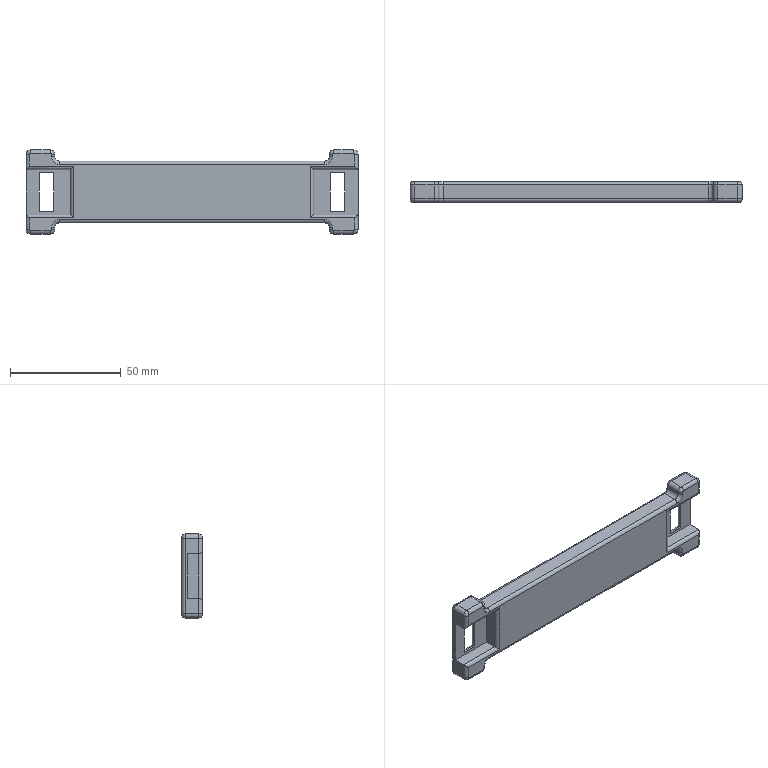Part | SolidWorks | features Extrusion 1, Fillet 1, ICE 1, MirrorPattern 1 | 1 solid | 106 faces | box 150 x 9.3 x 38 mm | volume 34912 mm3 | cylinder 52 | plane 30 | torus 24 | commonest cylinder face diameters 3 x40 4 x12